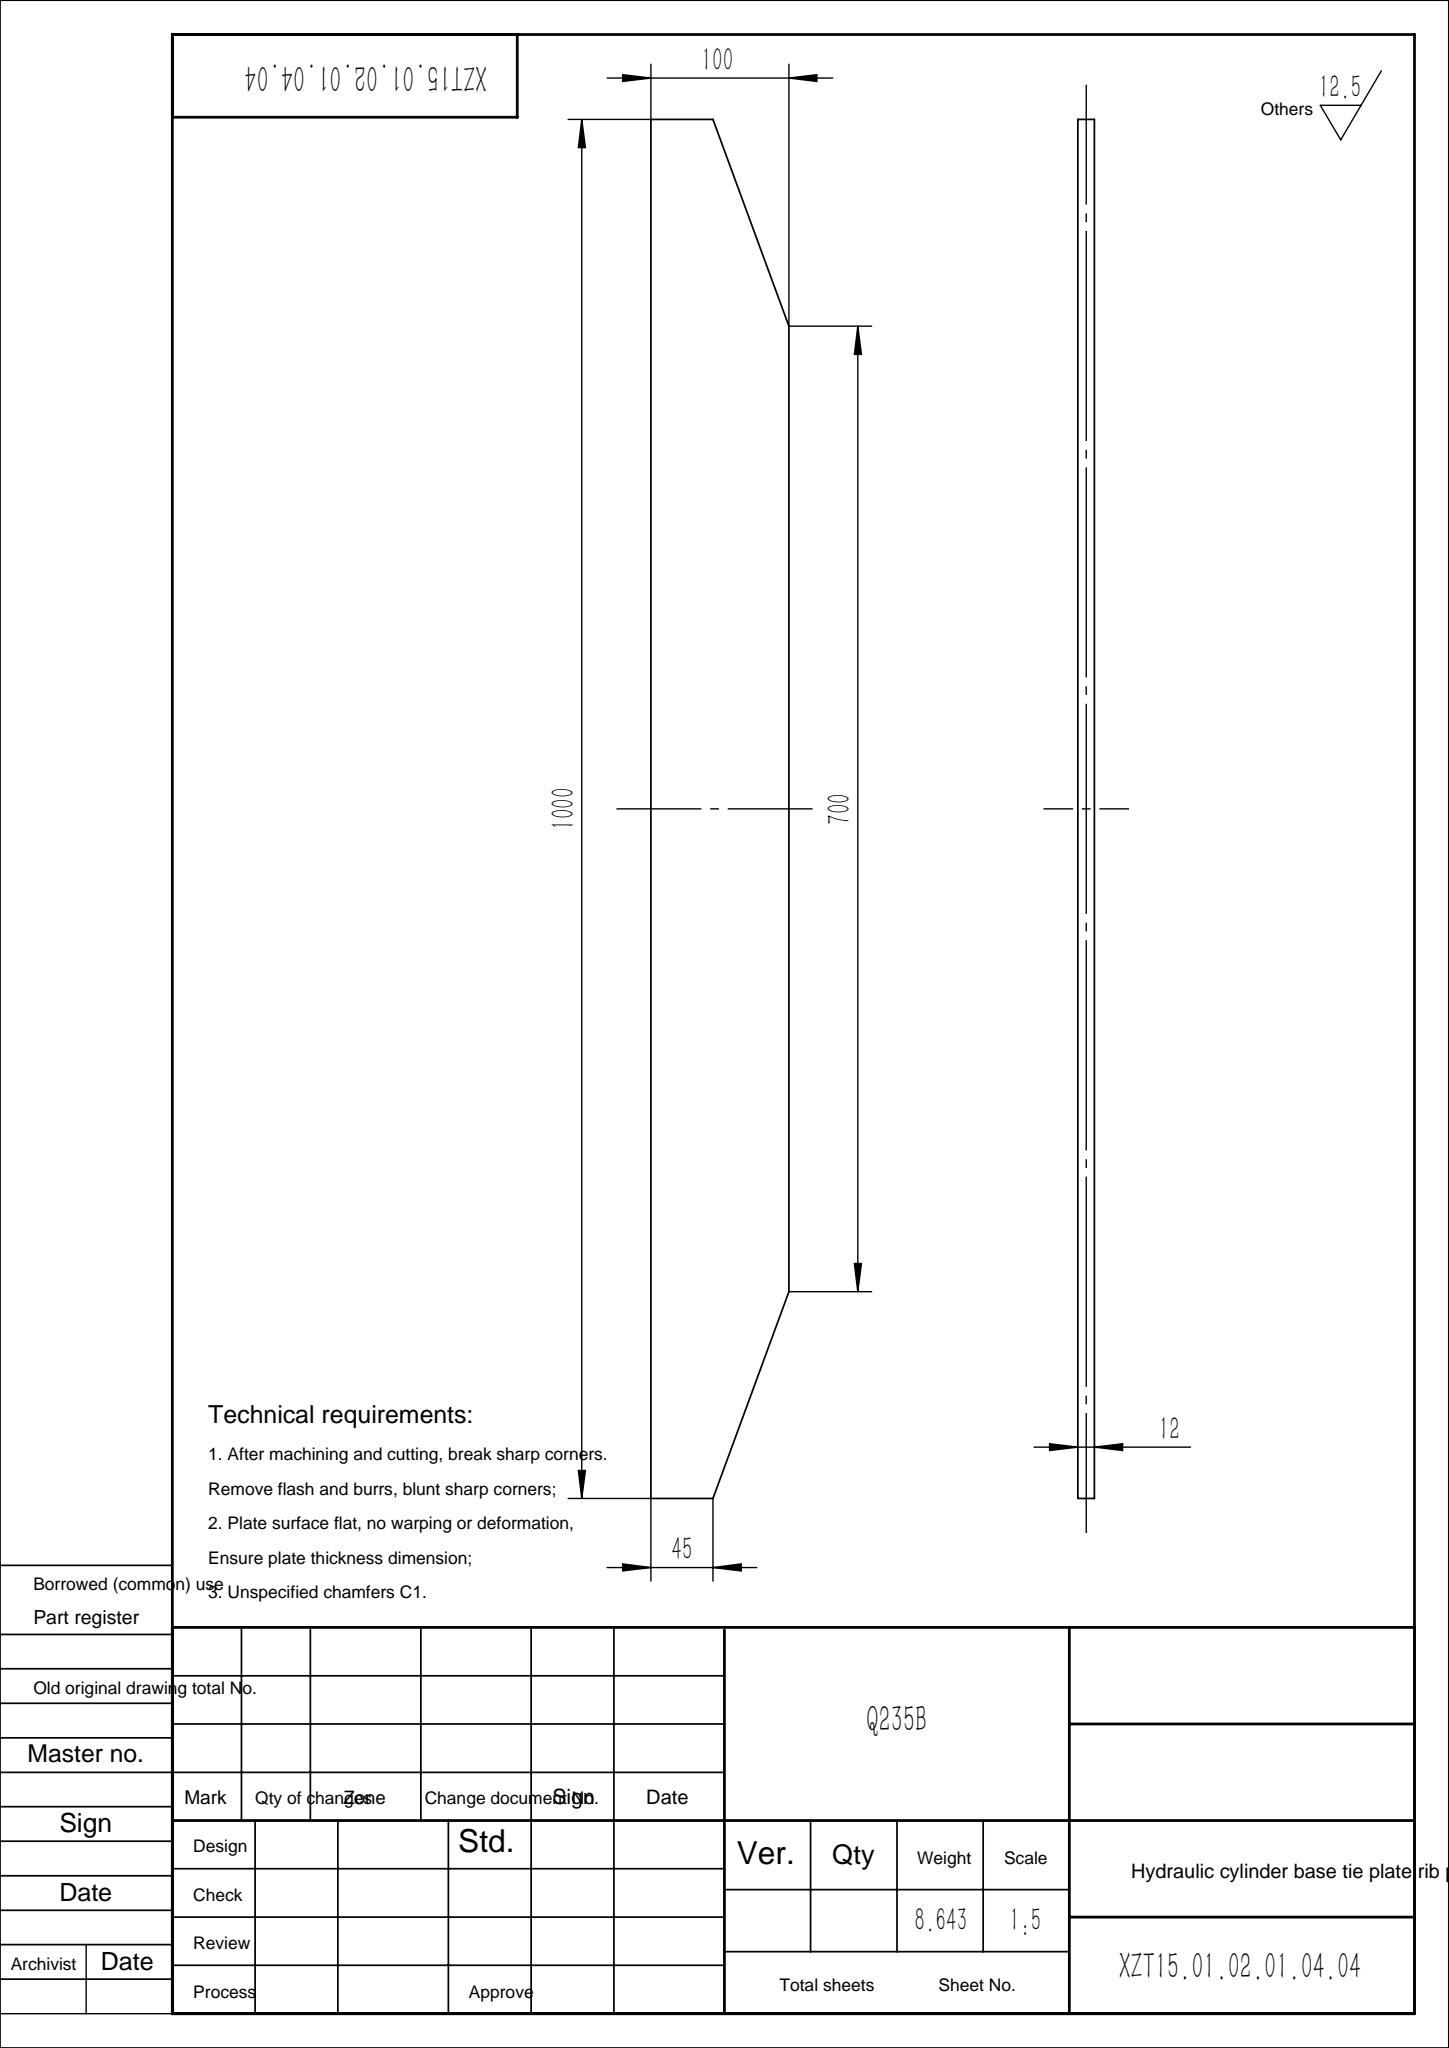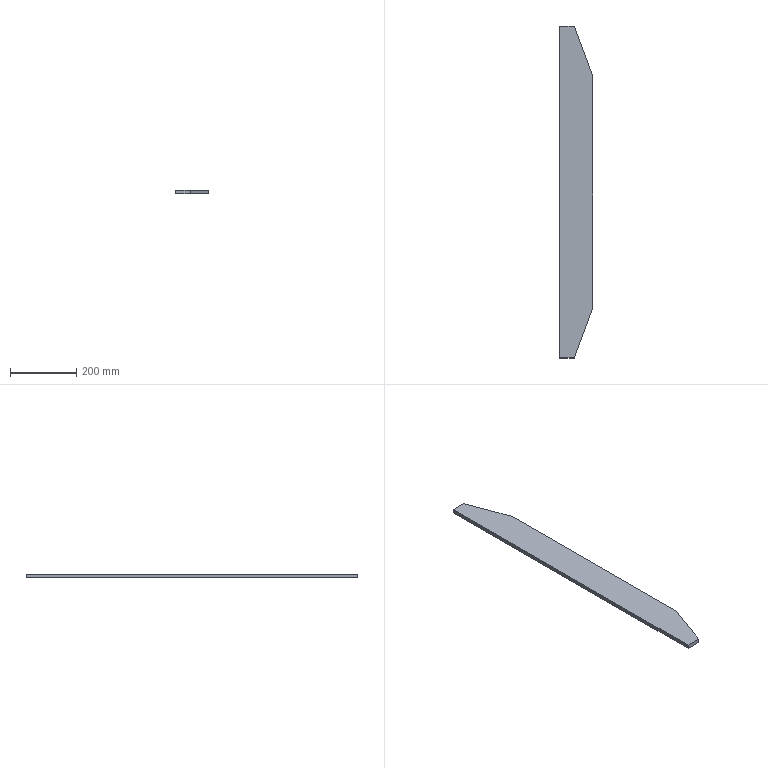Part | SolidWorks | features Extrusion 1 | 1 solid | 8 faces | box 100 x 1000 x 12 mm | volume 1101000 mm3 | plane 8
STEP:
#1=CARTESIAN_POINT('',(45.,500.,-6.));
#2=VERTEX_POINT('',#1);
#3=CARTESIAN_POINT('',(0.,500.,-6.));
#4=VERTEX_POINT('',#3);
#5=CARTESIAN_POINT('',(0.,500.,-6.));
#6=DIRECTION('',(-1.,0.,0.));
#7=VECTOR('',#6,1000.);
#8=LINE('',#5,#7);
#9=EDGE_CURVE('',#2,#4,#8,.T.);
#10=ORIENTED_EDGE('',*,*,#9,.T.);
#11=CARTESIAN_POINT('',(0.,500.,6.));
#12=VERTEX_POINT('',#11);
#13=CARTESIAN_POINT('',(0.,500.,6.));
#14=DIRECTION('',(0.,0.,-1.));
#15=VECTOR('',#14,1000.);
#16=LINE('',#13,#15);
#17=EDGE_CURVE('',#12,#4,#16,.T.);
#18=ORIENTED_EDGE('',*,*,#17,.F.);
#19=CARTESIAN_POINT('',(45.,500.,6.));
#20=VERTEX_POINT('',#19);
#21=CARTESIAN_POINT('',(0.,500.,6.));
#22=DIRECTION('',(-1.,0.,0.));
#23=VECTOR('',#22,1000.);
#24=LINE('',#21,#23);
#25=EDGE_CURVE('',#20,#12,#24,.T.);
#26=ORIENTED_EDGE('',*,*,#25,.F.);
#27=CARTESIAN_POINT('',(45.,500.,6.));
#28=DIRECTION('',(0.,0.,-1.));
#29=VECTOR('',#28,1000.);
#30=LINE('',#27,#29);
#31=EDGE_CURVE('',#20,#2,#30,.T.);
#32=ORIENTED_EDGE('',*,*,#31,.T.);
#33=EDGE_LOOP('',(#10,#18,#26,#32));
#34=FACE_OUTER_BOUND('',#33,.T.);
#35=CARTESIAN_POINT('',(0.,500.,6.));
#36=DIRECTION('',(0.,-1.,0.));
#37=DIRECTION('',(0.,0.,-1.));
#38=AXIS2_PLACEMENT_3D('',#35,#36,#37);
#39=PLANE('',#38);
#40=ADVANCED_FACE('',(#34),#39,.F.);
#41=CARTESIAN_POINT('',(0.,-500.,-6.));
#42=VERTEX_POINT('',#41);
#43=CARTESIAN_POINT('',(0.,-500.,-6.));
#44=DIRECTION('',(0.,-1.,0.));
#45=VECTOR('',#44,1000.);
#46=LINE('',#43,#45);
#47=EDGE_CURVE('',#4,#42,#46,.T.);
#48=ORIENTED_EDGE('',*,*,#47,.T.);
#49=CARTESIAN_POINT('',(0.,-500.,6.));
#50=VERTEX_POINT('',#49);
#51=CARTESIAN_POINT('',(0.,-500.,6.));
#52=DIRECTION('',(0.,0.,-1.));
#53=VECTOR('',#52,1000.);
#54=LINE('',#51,#53);
#55=EDGE_CURVE('',#50,#42,#54,.T.);
#56=ORIENTED_EDGE('',*,*,#55,.F.);
#57=CARTESIAN_POINT('',(0.,-500.,6.));
#58=DIRECTION('',(0.,-1.,0.));
#59=VECTOR('',#58,1000.);
#60=LINE('',#57,#59);
#61=EDGE_CURVE('',#12,#50,#60,.T.);
#62=ORIENTED_EDGE('',*,*,#61,.F.);
#63=ORIENTED_EDGE('',*,*,#17,.T.);
#64=EDGE_LOOP('',(#48,#56,#62,#63));
#65=FACE_OUTER_BOUND('',#64,.T.);
#66=CARTESIAN_POINT('',(0.,-500.,6.));
#67=DIRECTION('',(1.,0.,0.));
#68=DIRECTION('',(0.,1.,0.));
#69=AXIS2_PLACEMENT_3D('',#66,#67,#68);
#70=PLANE('',#69);
#71=ADVANCED_FACE('',(#65),#70,.F.);
#72=CARTESIAN_POINT('',(45.,-500.,-6.));
#73=VERTEX_POINT('',#72);
#74=CARTESIAN_POINT('',(0.,-500.,-6.));
#75=DIRECTION('',(1.,0.,0.));
#76=VECTOR('',#75,1000.);
#77=LINE('',#74,#76);
#78=EDGE_CURVE('',#42,#73,#77,.T.);
#79=ORIENTED_EDGE('',*,*,#78,.T.);
#80=CARTESIAN_POINT('',(45.,-500.,6.));
#81=VERTEX_POINT('',#80);
#82=CARTESIAN_POINT('',(45.,-500.,6.));
#83=DIRECTION('',(0.,0.,-1.));
#84=VECTOR('',#83,1000.);
#85=LINE('',#82,#84);
#86=EDGE_CURVE('',#81,#73,#85,.T.);
#87=ORIENTED_EDGE('',*,*,#86,.F.);
#88=CARTESIAN_POINT('',(0.,-500.,6.));
#89=DIRECTION('',(1.,0.,0.));
#90=VECTOR('',#89,1000.);
#91=LINE('',#88,#90);
#92=EDGE_CURVE('',#50,#81,#91,.T.);
#93=ORIENTED_EDGE('',*,*,#92,.F.);
#94=ORIENTED_EDGE('',*,*,#55,.T.);
#95=EDGE_LOOP('',(#79,#87,#93,#94));
#96=FACE_OUTER_BOUND('',#95,.T.);
#97=CARTESIAN_POINT('',(0.,-500.,6.));
#98=DIRECTION('',(0.,1.,0.));
#99=DIRECTION('',(0.,0.,1.));
#100=AXIS2_PLACEMENT_3D('',#97,#98,#99);
#101=PLANE('',#100);
#102=ADVANCED_FACE('',(#96),#101,.F.);
#103=CARTESIAN_POINT('',(100.,-350.,-6.));
#104=VERTEX_POINT('',#103);
#105=CARTESIAN_POINT('',(45.,-500.,-6.));
#106=DIRECTION('',(0.3443,0.9389,0.));
#107=VECTOR('',#106,1000.);
#108=LINE('',#105,#107);
#109=EDGE_CURVE('',#73,#104,#108,.T.);
#110=ORIENTED_EDGE('',*,*,#109,.T.);
#111=CARTESIAN_POINT('',(100.,-350.,6.));
#112=VERTEX_POINT('',#111);
#113=CARTESIAN_POINT('',(100.,-350.,6.));
#114=DIRECTION('',(0.,0.,-1.));
#115=VECTOR('',#114,1000.);
#116=LINE('',#113,#115);
#117=EDGE_CURVE('',#112,#104,#116,.T.);
#118=ORIENTED_EDGE('',*,*,#117,.F.);
#119=CARTESIAN_POINT('',(45.,-500.,6.));
#120=DIRECTION('',(0.3443,0.9389,0.));
#121=VECTOR('',#120,1000.);
#122=LINE('',#119,#121);
#123=EDGE_CURVE('',#81,#112,#122,.T.);
#124=ORIENTED_EDGE('',*,*,#123,.F.);
#125=ORIENTED_EDGE('',*,*,#86,.T.);
#126=EDGE_LOOP('',(#110,#118,#124,#125));
#127=FACE_OUTER_BOUND('',#126,.T.);
#128=CARTESIAN_POINT('',(45.,-500.,6.));
#129=DIRECTION('',(-0.9389,0.3443,0.));
#130=DIRECTION('',(-0.3443,-0.9389,0.));
#131=AXIS2_PLACEMENT_3D('',#128,#129,#130);
#132=PLANE('',#131);
#133=ADVANCED_FACE('',(#127),#132,.F.);
#134=CARTESIAN_POINT('',(100.,350.,-6.));
#135=VERTEX_POINT('',#134);
#136=CARTESIAN_POINT('',(100.,350.,-6.));
#137=DIRECTION('',(0.,1.,0.));
#138=VECTOR('',#137,1000.);
#139=LINE('',#136,#138);
#140=EDGE_CURVE('',#104,#135,#139,.T.);
#141=ORIENTED_EDGE('',*,*,#140,.T.);
#142=CARTESIAN_POINT('',(100.,350.,6.));
#143=VERTEX_POINT('',#142);
#144=CARTESIAN_POINT('',(100.,350.,6.));
#145=DIRECTION('',(0.,0.,-1.));
#146=VECTOR('',#145,1000.);
#147=LINE('',#144,#146);
#148=EDGE_CURVE('',#143,#135,#147,.T.);
#149=ORIENTED_EDGE('',*,*,#148,.F.);
#150=CARTESIAN_POINT('',(100.,350.,6.));
#151=DIRECTION('',(0.,1.,0.));
#152=VECTOR('',#151,1000.);
#153=LINE('',#150,#152);
#154=EDGE_CURVE('',#112,#143,#153,.T.);
#155=ORIENTED_EDGE('',*,*,#154,.F.);
#156=ORIENTED_EDGE('',*,*,#117,.T.);
#157=EDGE_LOOP('',(#141,#149,#155,#156));
#158=FACE_OUTER_BOUND('',#157,.T.);
#159=CARTESIAN_POINT('',(100.,350.,6.));
#160=DIRECTION('',(-1.,0.,0.));
#161=DIRECTION('',(0.,-1.,0.));
#162=AXIS2_PLACEMENT_3D('',#159,#160,#161);
#163=PLANE('',#162);
#164=ADVANCED_FACE('',(#158),#163,.F.);
#165=CARTESIAN_POINT('',(45.,500.,-6.));
#166=DIRECTION('',(-0.3443,0.9389,0.));
#167=VECTOR('',#166,1000.);
#168=LINE('',#165,#167);
#169=EDGE_CURVE('',#135,#2,#168,.T.);
#170=ORIENTED_EDGE('',*,*,#169,.T.);
#171=ORIENTED_EDGE('',*,*,#31,.F.);
#172=CARTESIAN_POINT('',(45.,500.,6.));
#173=DIRECTION('',(-0.3443,0.9389,0.));
#174=VECTOR('',#173,1000.);
#175=LINE('',#172,#174);
#176=EDGE_CURVE('',#143,#20,#175,.T.);
#177=ORIENTED_EDGE('',*,*,#176,.F.);
#178=ORIENTED_EDGE('',*,*,#148,.T.);
#179=EDGE_LOOP('',(#170,#171,#177,#178));
#180=FACE_OUTER_BOUND('',#179,.T.);
#181=CARTESIAN_POINT('',(45.,500.,6.));
#182=DIRECTION('',(-0.9389,-0.3443,0.));
#183=DIRECTION('',(0.3443,-0.9389,0.));
#184=AXIS2_PLACEMENT_3D('',#181,#182,#183);
#185=PLANE('',#184);
#186=ADVANCED_FACE('',(#180),#185,.F.);
#187=ORIENTED_EDGE('',*,*,#25,.T.);
#188=ORIENTED_EDGE('',*,*,#61,.T.);
#189=ORIENTED_EDGE('',*,*,#92,.T.);
#190=ORIENTED_EDGE('',*,*,#123,.T.);
#191=ORIENTED_EDGE('',*,*,#154,.T.);
#192=ORIENTED_EDGE('',*,*,#176,.T.);
#193=EDGE_LOOP('',(#187,#188,#189,#190,#191,#192));
#194=FACE_OUTER_BOUND('',#193,.T.);
#195=CARTESIAN_POINT('',(0.,0.,6.));
#196=DIRECTION('',(0.,0.,-1.));
#197=DIRECTION('',(-1.,0.,0.));
#198=AXIS2_PLACEMENT_3D('',#195,#196,#197);
#199=PLANE('',#198);
#200=ADVANCED_FACE('',(#194),#199,.F.);
#201=ORIENTED_EDGE('',*,*,#9,.F.);
#202=ORIENTED_EDGE('',*,*,#169,.F.);
#203=ORIENTED_EDGE('',*,*,#140,.F.);
#204=ORIENTED_EDGE('',*,*,#109,.F.);
#205=ORIENTED_EDGE('',*,*,#78,.F.);
#206=ORIENTED_EDGE('',*,*,#47,.F.);
#207=EDGE_LOOP('',(#201,#202,#203,#204,#205,#206));
#208=FACE_OUTER_BOUND('',#207,.T.);
#209=CARTESIAN_POINT('',(0.,0.,-6.));
#210=DIRECTION('',(0.,0.,-1.));
#211=DIRECTION('',(-1.,0.,0.));
#212=AXIS2_PLACEMENT_3D('',#209,#210,#211);
#213=PLANE('',#212);
#214=ADVANCED_FACE('',(#208),#213,.T.);
#215=CLOSED_SHELL('',(#40,#71,#102,#133,#164,#186,#200,#214));
#216=MANIFOLD_SOLID_BREP('',#215);
#217=CARTESIAN_POINT('',(0.,0.,0.));
#218=DIRECTION('',(0.,0.,1.));
#219=DIRECTION('',(1.,0.,0.));
#220=AXIS2_PLACEMENT_3D('',#217,#218,#219);
#221=(LENGTH_UNIT()NAMED_UNIT(*)SI_UNIT(.MILLI.,.METRE.));
#222=UNCERTAINTY_MEASURE_WITH_UNIT(LENGTH_MEASURE(0.00001),#221,'','');
#223=(NAMED_UNIT(*)PLANE_ANGLE_UNIT()SI_UNIT($,.RADIAN.));
#224=(NAMED_UNIT(*)SI_UNIT($,.STERADIAN.)SOLID_ANGLE_UNIT());
#225=(GEOMETRIC_REPRESENTATION_CONTEXT(3)GLOBAL_UNCERTAINTY_ASSIGNED_CONTEXT((#222))GLOBAL_UNIT_ASSIGNED_CONTEXT((#221,#223,#224))REPRESENTATION_CONTEXT('',''));
#226=ADVANCED_BREP_SHAPE_REPRESENTATION('',(#216,#220),#225);